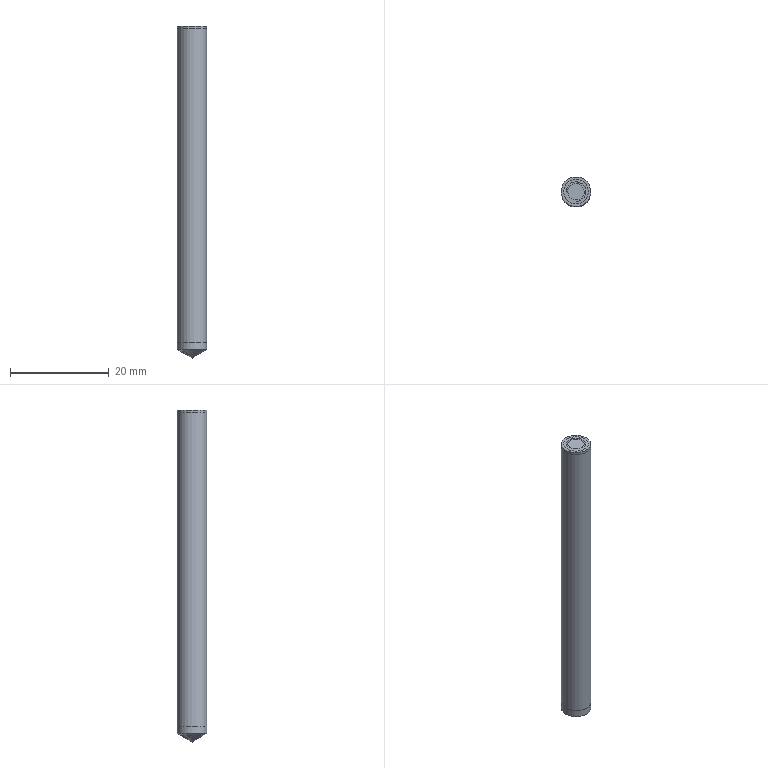Part | STEP file | EE030606500 | 2 solids | 45 faces | box 6 x 6 x 67.232 mm | volume 3615 mm3 | plane 15 | other 13 | cone 11 | cylinder 5 | torus 1 | commonest cylinder face diameters 6 x2 3.333 x1 3.987 x1 4 x1